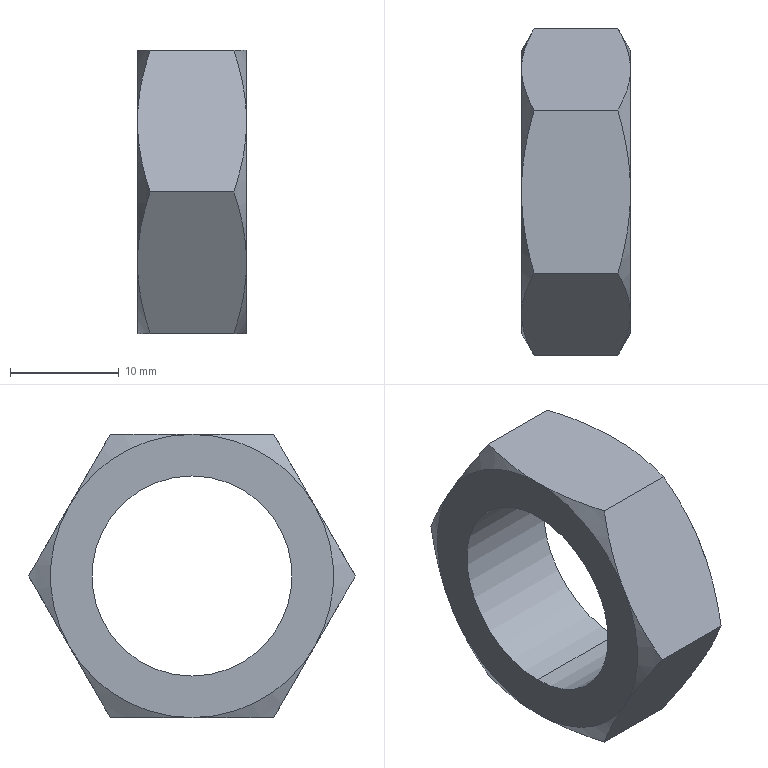Part | SolidWorks | features BaseBody 1 | 1 solid | 22 faces | box 10 x 30.022 x 26 mm | volume 3164 mm3 | cone 12 | plane 8 | cylinder 2 | commonest cylinder face diameters 18.376 x2
STEP:
#1=CARTESIAN_POINT('',(-65.,0.,9.188));
#2=VERTEX_POINT('',#1);
#3=CARTESIAN_POINT('',(-65.,0.,-9.188));
#4=VERTEX_POINT('',#3);
#5=CARTESIAN_POINT('',(-65.,0.,0.));
#6=DIRECTION('',(1.,0.,0.));
#7=DIRECTION('',(0.,0.,-1.));
#8=AXIS2_PLACEMENT_3D('',#5,#6,#7);
#9=CIRCLE('',#8,9.188);
#10=EDGE_CURVE('',#2,#4,#9,.T.);
#11=ORIENTED_EDGE('',*,*,#10,.F.);
#12=CARTESIAN_POINT('',(-55.,0.,9.188));
#13=VERTEX_POINT('',#12);
#14=CARTESIAN_POINT('',(-60.,0.,9.188));
#15=DIRECTION('',(1.,0.,0.));
#16=VECTOR('',#15,1000.);
#17=LINE('',#14,#16);
#18=EDGE_CURVE('',#2,#13,#17,.T.);
#19=ORIENTED_EDGE('',*,*,#18,.T.);
#20=CARTESIAN_POINT('',(-55.,0.,-9.188));
#21=VERTEX_POINT('',#20);
#22=CARTESIAN_POINT('',(-55.,0.,0.));
#23=DIRECTION('',(-1.,0.,0.));
#24=DIRECTION('',(0.,0.,-1.));
#25=AXIS2_PLACEMENT_3D('',#22,#23,#24);
#26=CIRCLE('',#25,9.188);
#27=EDGE_CURVE('',#21,#13,#26,.T.);
#28=ORIENTED_EDGE('',*,*,#27,.F.);
#29=CARTESIAN_POINT('',(-60.,0.,-9.188));
#30=DIRECTION('',(1.,0.,0.));
#31=VECTOR('',#30,1000.);
#32=LINE('',#29,#31);
#33=EDGE_CURVE('',#4,#21,#32,.T.);
#34=ORIENTED_EDGE('',*,*,#33,.F.);
#35=EDGE_LOOP('',(#11,#19,#28,#34));
#36=FACE_OUTER_BOUND('',#35,.T.);
#37=CARTESIAN_POINT('',(-60.,0.,0.));
#38=DIRECTION('',(1.,0.,0.));
#39=DIRECTION('',(0.,0.,-1.));
#40=AXIS2_PLACEMENT_3D('',#37,#38,#39);
#41=CYLINDRICAL_SURFACE('',#40,9.188);
#42=ADVANCED_FACE('',(#36),#41,.F.);
#43=ORIENTED_EDGE('',*,*,#18,.F.);
#44=CARTESIAN_POINT('',(-65.,0.,0.));
#45=DIRECTION('',(1.,0.,0.));
#46=DIRECTION('',(0.,0.,-1.));
#47=AXIS2_PLACEMENT_3D('',#44,#45,#46);
#48=CIRCLE('',#47,9.188);
#49=EDGE_CURVE('',#4,#2,#48,.T.);
#50=ORIENTED_EDGE('',*,*,#49,.F.);
#51=ORIENTED_EDGE('',*,*,#33,.T.);
#52=CARTESIAN_POINT('',(-55.,0.,0.));
#53=DIRECTION('',(-1.,0.,0.));
#54=DIRECTION('',(0.,0.,-1.));
#55=AXIS2_PLACEMENT_3D('',#52,#53,#54);
#56=CIRCLE('',#55,9.188);
#57=EDGE_CURVE('',#13,#21,#56,.T.);
#58=ORIENTED_EDGE('',*,*,#57,.F.);
#59=EDGE_LOOP('',(#43,#50,#51,#58));
#60=FACE_OUTER_BOUND('',#59,.T.);
#61=CARTESIAN_POINT('',(-60.,0.,0.));
#62=DIRECTION('',(1.,0.,0.));
#63=DIRECTION('',(0.,0.,-1.));
#64=AXIS2_PLACEMENT_3D('',#61,#62,#63);
#65=CYLINDRICAL_SURFACE('',#64,9.188);
#66=ADVANCED_FACE('',(#60),#65,.F.);
#67=ORIENTED_EDGE('',*,*,#27,.T.);
#68=ORIENTED_EDGE('',*,*,#57,.T.);
#69=EDGE_LOOP('',(#67,#68));
#70=FACE_BOUND('',#69,.T.);
#71=CARTESIAN_POINT('',(-55.,0.,13.));
#72=VERTEX_POINT('',#71);
#73=CARTESIAN_POINT('',(-55.,-11.258,6.5));
#74=VERTEX_POINT('',#73);
#75=CARTESIAN_POINT('',(-55.,0.,0.));
#76=DIRECTION('',(1.,0.,0.));
#77=DIRECTION('',(0.,0.,1.));
#78=AXIS2_PLACEMENT_3D('',#75,#76,#77);
#79=CIRCLE('',#78,13.);
#80=EDGE_CURVE('',#72,#74,#79,.T.);
#81=ORIENTED_EDGE('',*,*,#80,.T.);
#82=CARTESIAN_POINT('',(-55.,-11.258,-6.5));
#83=VERTEX_POINT('',#82);
#84=CARTESIAN_POINT('',(-55.,0.,0.));
#85=DIRECTION('',(1.,0.,0.));
#86=DIRECTION('',(0.,0.,1.));
#87=AXIS2_PLACEMENT_3D('',#84,#85,#86);
#88=CIRCLE('',#87,13.);
#89=EDGE_CURVE('',#74,#83,#88,.T.);
#90=ORIENTED_EDGE('',*,*,#89,.T.);
#91=CARTESIAN_POINT('',(-55.,0.,-13.));
#92=VERTEX_POINT('',#91);
#93=CARTESIAN_POINT('',(-55.,0.,0.));
#94=DIRECTION('',(1.,0.,0.));
#95=DIRECTION('',(0.,0.,1.));
#96=AXIS2_PLACEMENT_3D('',#93,#94,#95);
#97=CIRCLE('',#96,13.);
#98=EDGE_CURVE('',#83,#92,#97,.T.);
#99=ORIENTED_EDGE('',*,*,#98,.T.);
#100=CARTESIAN_POINT('',(-55.,11.258,-6.5));
#101=VERTEX_POINT('',#100);
#102=CARTESIAN_POINT('',(-55.,0.,0.));
#103=DIRECTION('',(1.,0.,0.));
#104=DIRECTION('',(0.,0.,1.));
#105=AXIS2_PLACEMENT_3D('',#102,#103,#104);
#106=CIRCLE('',#105,13.);
#107=EDGE_CURVE('',#92,#101,#106,.T.);
#108=ORIENTED_EDGE('',*,*,#107,.T.);
#109=CARTESIAN_POINT('',(-55.,11.258,6.5));
#110=VERTEX_POINT('',#109);
#111=CARTESIAN_POINT('',(-55.,0.,0.));
#112=DIRECTION('',(1.,0.,0.));
#113=DIRECTION('',(0.,0.,1.));
#114=AXIS2_PLACEMENT_3D('',#111,#112,#113);
#115=CIRCLE('',#114,13.);
#116=EDGE_CURVE('',#101,#110,#115,.T.);
#117=ORIENTED_EDGE('',*,*,#116,.T.);
#118=CARTESIAN_POINT('',(-55.,0.,0.));
#119=DIRECTION('',(1.,0.,0.));
#120=DIRECTION('',(0.,0.,1.));
#121=AXIS2_PLACEMENT_3D('',#118,#119,#120);
#122=CIRCLE('',#121,13.);
#123=EDGE_CURVE('',#110,#72,#122,.T.);
#124=ORIENTED_EDGE('',*,*,#123,.T.);
#125=EDGE_LOOP('',(#81,#90,#99,#108,#117,#124));
#126=FACE_OUTER_BOUND('',#125,.T.);
#127=CARTESIAN_POINT('',(-55.,-11.094,0.));
#128=DIRECTION('',(1.,0.,0.));
#129=DIRECTION('',(0.,0.,-1.));
#130=AXIS2_PLACEMENT_3D('',#127,#128,#129);
#131=PLANE('',#130);
#132=ADVANCED_FACE('',(#70,#126),#131,.T.);
#133=CARTESIAN_POINT('',(-65.,11.258,-6.5));
#134=VERTEX_POINT('',#133);
#135=CARTESIAN_POINT('',(-65.,0.,-13.));
#136=VERTEX_POINT('',#135);
#137=CARTESIAN_POINT('',(-65.,0.,0.));
#138=DIRECTION('',(-1.,0.,0.));
#139=DIRECTION('',(0.,0.,-1.));
#140=AXIS2_PLACEMENT_3D('',#137,#138,#139);
#141=CIRCLE('',#140,13.);
#142=EDGE_CURVE('',#134,#136,#141,.T.);
#143=ORIENTED_EDGE('',*,*,#142,.T.);
#144=CARTESIAN_POINT('',(-65.,-11.258,-6.5));
#145=VERTEX_POINT('',#144);
#146=CARTESIAN_POINT('',(-65.,0.,0.));
#147=DIRECTION('',(-1.,0.,0.));
#148=DIRECTION('',(0.,0.,-1.));
#149=AXIS2_PLACEMENT_3D('',#146,#147,#148);
#150=CIRCLE('',#149,13.);
#151=EDGE_CURVE('',#136,#145,#150,.T.);
#152=ORIENTED_EDGE('',*,*,#151,.T.);
#153=CARTESIAN_POINT('',(-65.,-11.258,6.5));
#154=VERTEX_POINT('',#153);
#155=CARTESIAN_POINT('',(-65.,0.,0.));
#156=DIRECTION('',(-1.,0.,0.));
#157=DIRECTION('',(0.,0.,-1.));
#158=AXIS2_PLACEMENT_3D('',#155,#156,#157);
#159=CIRCLE('',#158,13.);
#160=EDGE_CURVE('',#145,#154,#159,.T.);
#161=ORIENTED_EDGE('',*,*,#160,.T.);
#162=CARTESIAN_POINT('',(-65.,0.,13.));
#163=VERTEX_POINT('',#162);
#164=CARTESIAN_POINT('',(-65.,0.,0.));
#165=DIRECTION('',(-1.,0.,0.));
#166=DIRECTION('',(0.,0.,-1.));
#167=AXIS2_PLACEMENT_3D('',#164,#165,#166);
#168=CIRCLE('',#167,13.);
#169=EDGE_CURVE('',#154,#163,#168,.T.);
#170=ORIENTED_EDGE('',*,*,#169,.T.);
#171=CARTESIAN_POINT('',(-65.,11.258,6.5));
#172=VERTEX_POINT('',#171);
#173=CARTESIAN_POINT('',(-65.,0.,0.));
#174=DIRECTION('',(-1.,0.,0.));
#175=DIRECTION('',(0.,0.,-1.));
#176=AXIS2_PLACEMENT_3D('',#173,#174,#175);
#177=CIRCLE('',#176,13.);
#178=EDGE_CURVE('',#163,#172,#177,.T.);
#179=ORIENTED_EDGE('',*,*,#178,.T.);
#180=CARTESIAN_POINT('',(-65.,0.,0.));
#181=DIRECTION('',(-1.,0.,0.));
#182=DIRECTION('',(0.,0.,-1.));
#183=AXIS2_PLACEMENT_3D('',#180,#181,#182);
#184=CIRCLE('',#183,13.);
#185=EDGE_CURVE('',#172,#134,#184,.T.);
#186=ORIENTED_EDGE('',*,*,#185,.T.);
#187=EDGE_LOOP('',(#143,#152,#161,#170,#179,#186));
#188=FACE_OUTER_BOUND('',#187,.T.);
#189=ORIENTED_EDGE('',*,*,#49,.T.);
#190=ORIENTED_EDGE('',*,*,#10,.T.);
#191=EDGE_LOOP('',(#189,#190));
#192=FACE_BOUND('',#191,.T.);
#193=CARTESIAN_POINT('',(-65.,-11.094,0.));
#194=DIRECTION('',(-1.,0.,0.));
#195=DIRECTION('',(0.,0.,1.));
#196=AXIS2_PLACEMENT_3D('',#193,#194,#195);
#197=PLANE('',#196);
#198=ADVANCED_FACE('',(#188,#192),#197,.T.);
#199=ORIENTED_EDGE('',*,*,#89,.F.);
#200=CARTESIAN_POINT('',(-56.161,-15.011,0.));
#201=VERTEX_POINT('',#200);
#202=CARTESIAN_POINT('',(-55.,-11.258,6.5));
#203=CARTESIAN_POINT('',(-55.,-11.899,5.391));
#204=CARTESIAN_POINT('',(-55.111,-12.531,4.296));
#205=CARTESIAN_POINT('',(-55.515,-13.78,2.132));
#206=CARTESIAN_POINT('',(-55.807,-14.398,1.062));
#207=CARTESIAN_POINT('',(-56.161,-15.011,0.));
#208=B_SPLINE_CURVE_WITH_KNOTS('',3,(#202,#203,#204,#205,#206,#207),.UNSPECIFIED.,.F.,.F.,(4,2,4),(0.,0.003797,0.007595),.UNSPECIFIED.);
#209=EDGE_CURVE('',#74,#201,#208,.T.);
#210=ORIENTED_EDGE('',*,*,#209,.T.);
#211=CARTESIAN_POINT('',(-56.161,-15.011,0.));
#212=CARTESIAN_POINT('',(-55.807,-14.398,-1.062));
#213=CARTESIAN_POINT('',(-55.515,-13.78,-2.132));
#214=CARTESIAN_POINT('',(-55.111,-12.531,-4.296));
#215=CARTESIAN_POINT('',(-55.,-11.899,-5.391));
#216=CARTESIAN_POINT('',(-55.,-11.258,-6.5));
#217=B_SPLINE_CURVE_WITH_KNOTS('',3,(#211,#212,#213,#214,#215,#216),.UNSPECIFIED.,.F.,.F.,(4,2,4),(0.,0.003797,0.007595),.UNSPECIFIED.);
#218=EDGE_CURVE('',#201,#83,#217,.T.);
#219=ORIENTED_EDGE('',*,*,#218,.T.);
#220=EDGE_LOOP('',(#199,#210,#219));
#221=FACE_OUTER_BOUND('',#220,.T.);
#222=CARTESIAN_POINT('',(-56.168,0.,0.));
#223=DIRECTION('',(-1.,0.,0.));
#224=DIRECTION('',(0.,0.,1.));
#225=AXIS2_PLACEMENT_3D('',#222,#223,#224);
#226=CONICAL_SURFACE('',#225,15.023,1.047);
#227=ADVANCED_FACE('',(#221),#226,.T.);
#228=CARTESIAN_POINT('',(-56.161,-7.506,13.));
#229=VERTEX_POINT('',#228);
#230=CARTESIAN_POINT('',(-56.161,-7.506,13.));
#231=CARTESIAN_POINT('',(-55.807,-8.119,11.938));
#232=CARTESIAN_POINT('',(-55.515,-8.736,10.868));
#233=CARTESIAN_POINT('',(-55.111,-9.986,8.704));
#234=CARTESIAN_POINT('',(-55.,-10.618,7.609));
#235=CARTESIAN_POINT('',(-55.,-11.258,6.5));
#236=B_SPLINE_CURVE_WITH_KNOTS('',3,(#230,#231,#232,#233,#234,#235),.UNSPECIFIED.,.F.,.F.,(4,2,4),(0.,0.003797,0.007595),.UNSPECIFIED.);
#237=EDGE_CURVE('',#229,#74,#236,.T.);
#238=ORIENTED_EDGE('',*,*,#237,.T.);
#239=ORIENTED_EDGE('',*,*,#80,.F.);
#240=CARTESIAN_POINT('',(-55.,0.,13.));
#241=CARTESIAN_POINT('',(-55.,-1.281,13.));
#242=CARTESIAN_POINT('',(-55.111,-2.545,13.));
#243=CARTESIAN_POINT('',(-55.515,-5.044,13.));
#244=CARTESIAN_POINT('',(-55.807,-6.279,13.));
#245=CARTESIAN_POINT('',(-56.161,-7.506,13.));
#246=B_SPLINE_CURVE_WITH_KNOTS('',3,(#240,#241,#242,#243,#244,#245),.UNSPECIFIED.,.F.,.F.,(4,2,4),(0.,0.003797,0.007595),.UNSPECIFIED.);
#247=EDGE_CURVE('',#72,#229,#246,.T.);
#248=ORIENTED_EDGE('',*,*,#247,.T.);
#249=EDGE_LOOP('',(#238,#239,#248));
#250=FACE_OUTER_BOUND('',#249,.T.);
#251=CARTESIAN_POINT('',(-56.168,0.,0.));
#252=DIRECTION('',(-1.,0.,0.));
#253=DIRECTION('',(0.,0.,1.));
#254=AXIS2_PLACEMENT_3D('',#251,#252,#253);
#255=CONICAL_SURFACE('',#254,15.023,1.047);
#256=ADVANCED_FACE('',(#250),#255,.T.);
#257=CARTESIAN_POINT('',(-56.161,7.506,13.));
#258=VERTEX_POINT('',#257);
#259=CARTESIAN_POINT('',(-56.161,7.506,13.));
#260=CARTESIAN_POINT('',(-55.807,6.279,13.));
#261=CARTESIAN_POINT('',(-55.515,5.044,13.));
#262=CARTESIAN_POINT('',(-55.111,2.545,13.));
#263=CARTESIAN_POINT('',(-55.,1.281,13.));
#264=CARTESIAN_POINT('',(-55.,0.,13.));
#265=B_SPLINE_CURVE_WITH_KNOTS('',3,(#259,#260,#261,#262,#263,#264),.UNSPECIFIED.,.F.,.F.,(4,2,4),(0.,0.003797,0.007595),.UNSPECIFIED.);
#266=EDGE_CURVE('',#258,#72,#265,.T.);
#267=ORIENTED_EDGE('',*,*,#266,.T.);
#268=ORIENTED_EDGE('',*,*,#123,.F.);
#269=CARTESIAN_POINT('',(-55.,11.258,6.5));
#270=CARTESIAN_POINT('',(-55.,10.618,7.609));
#271=CARTESIAN_POINT('',(-55.111,9.986,8.704));
#272=CARTESIAN_POINT('',(-55.515,8.736,10.868));
#273=CARTESIAN_POINT('',(-55.807,8.119,11.938));
#274=CARTESIAN_POINT('',(-56.161,7.506,13.));
#275=B_SPLINE_CURVE_WITH_KNOTS('',3,(#269,#270,#271,#272,#273,#274),.UNSPECIFIED.,.F.,.F.,(4,2,4),(0.,0.003797,0.007595),.UNSPECIFIED.);
#276=EDGE_CURVE('',#110,#258,#275,.T.);
#277=ORIENTED_EDGE('',*,*,#276,.T.);
#278=EDGE_LOOP('',(#267,#268,#277));
#279=FACE_OUTER_BOUND('',#278,.T.);
#280=CARTESIAN_POINT('',(-56.168,0.,0.));
#281=DIRECTION('',(-1.,0.,0.));
#282=DIRECTION('',(0.,0.,1.));
#283=AXIS2_PLACEMENT_3D('',#280,#281,#282);
#284=CONICAL_SURFACE('',#283,15.023,1.047);
#285=ADVANCED_FACE('',(#279),#284,.T.);
#286=CARTESIAN_POINT('',(-56.161,15.011,0.));
#287=VERTEX_POINT('',#286);
#288=CARTESIAN_POINT('',(-56.161,15.011,0.));
#289=CARTESIAN_POINT('',(-55.807,14.398,1.062));
#290=CARTESIAN_POINT('',(-55.515,13.78,2.132));
#291=CARTESIAN_POINT('',(-55.111,12.531,4.296));
#292=CARTESIAN_POINT('',(-55.,11.899,5.391));
#293=CARTESIAN_POINT('',(-55.,11.258,6.5));
#294=B_SPLINE_CURVE_WITH_KNOTS('',3,(#288,#289,#290,#291,#292,#293),.UNSPECIFIED.,.F.,.F.,(4,2,4),(0.,0.003797,0.007595),.UNSPECIFIED.);
#295=EDGE_CURVE('',#287,#110,#294,.T.);
#296=ORIENTED_EDGE('',*,*,#295,.T.);
#297=ORIENTED_EDGE('',*,*,#116,.F.);
#298=CARTESIAN_POINT('',(-55.,11.258,-6.5));
#299=CARTESIAN_POINT('',(-55.,11.899,-5.391));
#300=CARTESIAN_POINT('',(-55.111,12.531,-4.296));
#301=CARTESIAN_POINT('',(-55.515,13.78,-2.132));
#302=CARTESIAN_POINT('',(-55.807,14.398,-1.062));
#303=CARTESIAN_POINT('',(-56.161,15.011,0.));
#304=B_SPLINE_CURVE_WITH_KNOTS('',3,(#298,#299,#300,#301,#302,#303),.UNSPECIFIED.,.F.,.F.,(4,2,4),(0.,0.003797,0.007595),.UNSPECIFIED.);
#305=EDGE_CURVE('',#101,#287,#304,.T.);
#306=ORIENTED_EDGE('',*,*,#305,.T.);
#307=EDGE_LOOP('',(#296,#297,#306));
#308=FACE_OUTER_BOUND('',#307,.T.);
#309=CARTESIAN_POINT('',(-56.168,0.,0.));
#310=DIRECTION('',(-1.,0.,0.));
#311=DIRECTION('',(0.,0.,1.));
#312=AXIS2_PLACEMENT_3D('',#309,#310,#311);
#313=CONICAL_SURFACE('',#312,15.023,1.047);
#314=ADVANCED_FACE('',(#308),#313,.T.);
#315=ORIENTED_EDGE('',*,*,#107,.F.);
#316=CARTESIAN_POINT('',(-56.161,7.506,-13.));
#317=VERTEX_POINT('',#316);
#318=CARTESIAN_POINT('',(-55.,0.,-13.));
#319=CARTESIAN_POINT('',(-55.,1.281,-13.));
#320=CARTESIAN_POINT('',(-55.111,2.545,-13.));
#321=CARTESIAN_POINT('',(-55.515,5.044,-13.));
#322=CARTESIAN_POINT('',(-55.807,6.279,-13.));
#323=CARTESIAN_POINT('',(-56.161,7.506,-13.));
#324=B_SPLINE_CURVE_WITH_KNOTS('',3,(#318,#319,#320,#321,#322,#323),.UNSPECIFIED.,.F.,.F.,(4,2,4),(0.,0.003797,0.007595),.UNSPECIFIED.);
#325=EDGE_CURVE('',#92,#317,#324,.T.);
#326=ORIENTED_EDGE('',*,*,#325,.T.);
#327=CARTESIAN_POINT('',(-56.161,7.506,-13.));
#328=CARTESIAN_POINT('',(-55.807,8.119,-11.938));
#329=CARTESIAN_POINT('',(-55.515,8.736,-10.868));
#330=CARTESIAN_POINT('',(-55.111,9.986,-8.704));
#331=CARTESIAN_POINT('',(-55.,10.618,-7.609));
#332=CARTESIAN_POINT('',(-55.,11.258,-6.5));
#333=B_SPLINE_CURVE_WITH_KNOTS('',3,(#327,#328,#329,#330,#331,#332),.UNSPECIFIED.,.F.,.F.,(4,2,4),(0.,0.003797,0.007595),.UNSPECIFIED.);
#334=EDGE_CURVE('',#317,#101,#333,.T.);
#335=ORIENTED_EDGE('',*,*,#334,.T.);
#336=EDGE_LOOP('',(#315,#326,#335));
#337=FACE_OUTER_BOUND('',#336,.T.);
#338=CARTESIAN_POINT('',(-56.168,0.,0.));
#339=DIRECTION('',(-1.,0.,0.));
#340=DIRECTION('',(0.,0.,1.));
#341=AXIS2_PLACEMENT_3D('',#338,#339,#340);
#342=CONICAL_SURFACE('',#341,15.023,1.047);
#343=ADVANCED_FACE('',(#337),#342,.T.);
#344=ORIENTED_EDGE('',*,*,#98,.F.);
#345=CARTESIAN_POINT('',(-56.161,-7.506,-13.));
#346=VERTEX_POINT('',#345);
#347=CARTESIAN_POINT('',(-55.,-11.258,-6.5));
#348=CARTESIAN_POINT('',(-55.,-10.618,-7.609));
#349=CARTESIAN_POINT('',(-55.111,-9.986,-8.704));
#350=CARTESIAN_POINT('',(-55.515,-8.736,-10.868));
#351=CARTESIAN_POINT('',(-55.807,-8.119,-11.938));
#352=CARTESIAN_POINT('',(-56.161,-7.506,-13.));
#353=B_SPLINE_CURVE_WITH_KNOTS('',3,(#347,#348,#349,#350,#351,#352),.UNSPECIFIED.,.F.,.F.,(4,2,4),(0.,0.003797,0.007595),.UNSPECIFIED.);
#354=EDGE_CURVE('',#83,#346,#353,.T.);
#355=ORIENTED_EDGE('',*,*,#354,.T.);
#356=CARTESIAN_POINT('',(-56.161,-7.506,-13.));
#357=CARTESIAN_POINT('',(-55.807,-6.279,-13.));
#358=CARTESIAN_POINT('',(-55.515,-5.044,-13.));
#359=CARTESIAN_POINT('',(-55.111,-2.545,-13.));
#360=CARTESIAN_POINT('',(-55.,-1.281,-13.));
#361=CARTESIAN_POINT('',(-55.,0.,-13.));
#362=B_SPLINE_CURVE_WITH_KNOTS('',3,(#356,#357,#358,#359,#360,#361),.UNSPECIFIED.,.F.,.F.,(4,2,4),(0.,0.003797,0.007595),.UNSPECIFIED.);
#363=EDGE_CURVE('',#346,#92,#362,.T.);
#364=ORIENTED_EDGE('',*,*,#363,.T.);
#365=EDGE_LOOP('',(#344,#355,#364));
#366=FACE_OUTER_BOUND('',#365,.T.);
#367=CARTESIAN_POINT('',(-56.168,0.,0.));
#368=DIRECTION('',(-1.,0.,0.));
#369=DIRECTION('',(0.,0.,1.));
#370=AXIS2_PLACEMENT_3D('',#367,#368,#369);
#371=CONICAL_SURFACE('',#370,15.023,1.047);
#372=ADVANCED_FACE('',(#366),#371,.T.);
#373=CARTESIAN_POINT('',(-63.839,-7.506,-13.));
#374=VERTEX_POINT('',#373);
#375=CARTESIAN_POINT('',(-63.839,-7.506,-13.));
#376=CARTESIAN_POINT('',(-64.193,-8.119,-11.938));
#377=CARTESIAN_POINT('',(-64.485,-8.736,-10.868));
#378=CARTESIAN_POINT('',(-64.889,-9.986,-8.704));
#379=CARTESIAN_POINT('',(-65.,-10.618,-7.609));
#380=CARTESIAN_POINT('',(-65.,-11.258,-6.5));
#381=B_SPLINE_CURVE_WITH_KNOTS('',3,(#375,#376,#377,#378,#379,#380),.UNSPECIFIED.,.F.,.F.,(4,2,4),(0.,0.003797,0.007595),.UNSPECIFIED.);
#382=EDGE_CURVE('',#374,#145,#381,.T.);
#383=ORIENTED_EDGE('',*,*,#382,.T.);
#384=ORIENTED_EDGE('',*,*,#151,.F.);
#385=CARTESIAN_POINT('',(-65.,0.,-13.));
#386=CARTESIAN_POINT('',(-65.,-1.281,-13.));
#387=CARTESIAN_POINT('',(-64.889,-2.545,-13.));
#388=CARTESIAN_POINT('',(-64.485,-5.044,-13.));
#389=CARTESIAN_POINT('',(-64.193,-6.279,-13.));
#390=CARTESIAN_POINT('',(-63.839,-7.506,-13.));
#391=B_SPLINE_CURVE_WITH_KNOTS('',3,(#385,#386,#387,#388,#389,#390),.UNSPECIFIED.,.F.,.F.,(4,2,4),(0.,0.003797,0.007595),.UNSPECIFIED.);
#392=EDGE_CURVE('',#136,#374,#391,.T.);
#393=ORIENTED_EDGE('',*,*,#392,.T.);
#394=EDGE_LOOP('',(#383,#384,#393));
#395=FACE_OUTER_BOUND('',#394,.T.);
#396=CARTESIAN_POINT('',(-63.832,0.,0.));
#397=DIRECTION('',(1.,0.,0.));
#398=DIRECTION('',(0.,0.,-1.));
#399=AXIS2_PLACEMENT_3D('',#396,#397,#398);
#400=CONICAL_SURFACE('',#399,15.023,1.047);
#401=ADVANCED_FACE('',(#395),#400,.T.);
#402=ORIENTED_EDGE('',*,*,#142,.F.);
#403=CARTESIAN_POINT('',(-63.839,7.506,-13.));
#404=VERTEX_POINT('',#403);
#405=CARTESIAN_POINT('',(-65.,11.258,-6.5));
#406=CARTESIAN_POINT('',(-65.,10.618,-7.609));
#407=CARTESIAN_POINT('',(-64.889,9.986,-8.704));
#408=CARTESIAN_POINT('',(-64.485,8.736,-10.868));
#409=CARTESIAN_POINT('',(-64.193,8.119,-11.938));
#410=CARTESIAN_POINT('',(-63.839,7.506,-13.));
#411=B_SPLINE_CURVE_WITH_KNOTS('',3,(#405,#406,#407,#408,#409,#410),.UNSPECIFIED.,.F.,.F.,(4,2,4),(0.,0.003797,0.007595),.UNSPECIFIED.);
#412=EDGE_CURVE('',#134,#404,#411,.T.);
#413=ORIENTED_EDGE('',*,*,#412,.T.);
#414=CARTESIAN_POINT('',(-63.839,7.506,-13.));
#415=CARTESIAN_POINT('',(-64.193,6.279,-13.));
#416=CARTESIAN_POINT('',(-64.485,5.044,-13.));
#417=CARTESIAN_POINT('',(-64.889,2.545,-13.));
#418=CARTESIAN_POINT('',(-65.,1.281,-13.));
#419=CARTESIAN_POINT('',(-65.,0.,-13.));
#420=B_SPLINE_CURVE_WITH_KNOTS('',3,(#414,#415,#416,#417,#418,#419),.UNSPECIFIED.,.F.,.F.,(4,2,4),(0.,0.003797,0.007595),.UNSPECIFIED.);
#421=EDGE_CURVE('',#404,#136,#420,.T.);
#422=ORIENTED_EDGE('',*,*,#421,.T.);
#423=EDGE_LOOP('',(#402,#413,#422));
#424=FACE_OUTER_BOUND('',#423,.T.);
#425=CARTESIAN_POINT('',(-63.832,0.,0.));
#426=DIRECTION('',(1.,0.,0.));
#427=DIRECTION('',(0.,0.,-1.));
#428=AXIS2_PLACEMENT_3D('',#425,#426,#427);
#429=CONICAL_SURFACE('',#428,15.023,1.047);
#430=ADVANCED_FACE('',(#424),#429,.T.);
#431=CARTESIAN_POINT('',(-63.839,15.011,0.));
#432=VERTEX_POINT('',#431);
#433=CARTESIAN_POINT('',(-63.839,15.011,0.));
#434=CARTESIAN_POINT('',(-64.193,14.398,-1.062));
#435=CARTESIAN_POINT('',(-64.485,13.78,-2.132));
#436=CARTESIAN_POINT('',(-64.889,12.531,-4.296));
#437=CARTESIAN_POINT('',(-65.,11.899,-5.391));
#438=CARTESIAN_POINT('',(-65.,11.258,-6.5));
#439=B_SPLINE_CURVE_WITH_KNOTS('',3,(#433,#434,#435,#436,#437,#438),.UNSPECIFIED.,.F.,.F.,(4,2,4),(0.,0.003797,0.007595),.UNSPECIFIED.);
#440=EDGE_CURVE('',#432,#134,#439,.T.);
#441=ORIENTED_EDGE('',*,*,#440,.T.);
#442=ORIENTED_EDGE('',*,*,#185,.F.);
#443=CARTESIAN_POINT('',(-65.,11.258,6.5));
#444=CARTESIAN_POINT('',(-65.,11.899,5.391));
#445=CARTESIAN_POINT('',(-64.889,12.531,4.296));
#446=CARTESIAN_POINT('',(-64.485,13.78,2.132));
#447=CARTESIAN_POINT('',(-64.193,14.398,1.062));
#448=CARTESIAN_POINT('',(-63.839,15.011,0.));
#449=B_SPLINE_CURVE_WITH_KNOTS('',3,(#443,#444,#445,#446,#447,#448),.UNSPECIFIED.,.F.,.F.,(4,2,4),(0.,0.003797,0.007595),.UNSPECIFIED.);
#450=EDGE_CURVE('',#172,#432,#449,.T.);
#451=ORIENTED_EDGE('',*,*,#450,.T.);
#452=EDGE_LOOP('',(#441,#442,#451));
#453=FACE_OUTER_BOUND('',#452,.T.);
#454=CARTESIAN_POINT('',(-63.832,0.,0.));
#455=DIRECTION('',(1.,0.,0.));
#456=DIRECTION('',(0.,0.,-1.));
#457=AXIS2_PLACEMENT_3D('',#454,#455,#456);
#458=CONICAL_SURFACE('',#457,15.023,1.047);
#459=ADVANCED_FACE('',(#453),#458,.T.);
#460=ORIENTED_EDGE('',*,*,#178,.F.);
#461=CARTESIAN_POINT('',(-63.839,7.506,13.));
#462=VERTEX_POINT('',#461);
#463=CARTESIAN_POINT('',(-65.,0.,13.));
#464=CARTESIAN_POINT('',(-65.,1.281,13.));
#465=CARTESIAN_POINT('',(-64.889,2.545,13.));
#466=CARTESIAN_POINT('',(-64.485,5.044,13.));
#467=CARTESIAN_POINT('',(-64.193,6.279,13.));
#468=CARTESIAN_POINT('',(-63.839,7.506,13.));
#469=B_SPLINE_CURVE_WITH_KNOTS('',3,(#463,#464,#465,#466,#467,#468),.UNSPECIFIED.,.F.,.F.,(4,2,4),(0.,0.003797,0.007595),.UNSPECIFIED.);
#470=EDGE_CURVE('',#163,#462,#469,.T.);
#471=ORIENTED_EDGE('',*,*,#470,.T.);
#472=CARTESIAN_POINT('',(-63.839,7.506,13.));
#473=CARTESIAN_POINT('',(-64.193,8.119,11.938));
#474=CARTESIAN_POINT('',(-64.485,8.736,10.868));
#475=CARTESIAN_POINT('',(-64.889,9.986,8.704));
#476=CARTESIAN_POINT('',(-65.,10.618,7.609));
#477=CARTESIAN_POINT('',(-65.,11.258,6.5));
#478=B_SPLINE_CURVE_WITH_KNOTS('',3,(#472,#473,#474,#475,#476,#477),.UNSPECIFIED.,.F.,.F.,(4,2,4),(0.,0.003797,0.007595),.UNSPECIFIED.);
#479=EDGE_CURVE('',#462,#172,#478,.T.);
#480=ORIENTED_EDGE('',*,*,#479,.T.);
#481=EDGE_LOOP('',(#460,#471,#480));
#482=FACE_OUTER_BOUND('',#481,.T.);
#483=CARTESIAN_POINT('',(-63.832,0.,0.));
#484=DIRECTION('',(1.,0.,0.));
#485=DIRECTION('',(0.,0.,-1.));
#486=AXIS2_PLACEMENT_3D('',#483,#484,#485);
#487=CONICAL_SURFACE('',#486,15.023,1.047);
#488=ADVANCED_FACE('',(#482),#487,.T.);
#489=CARTESIAN_POINT('',(-63.839,-7.506,13.));
#490=VERTEX_POINT('',#489);
#491=CARTESIAN_POINT('',(-63.839,-7.506,13.));
#492=CARTESIAN_POINT('',(-64.193,-6.279,13.));
#493=CARTESIAN_POINT('',(-64.485,-5.044,13.));
#494=CARTESIAN_POINT('',(-64.889,-2.545,13.));
#495=CARTESIAN_POINT('',(-65.,-1.281,13.));
#496=CARTESIAN_POINT('',(-65.,0.,13.));
#497=B_SPLINE_CURVE_WITH_KNOTS('',3,(#491,#492,#493,#494,#495,#496),.UNSPECIFIED.,.F.,.F.,(4,2,4),(0.,0.003797,0.007595),.UNSPECIFIED.);
#498=EDGE_CURVE('',#490,#163,#497,.T.);
#499=ORIENTED_EDGE('',*,*,#498,.T.);
#500=ORIENTED_EDGE('',*,*,#169,.F.);
#501=CARTESIAN_POINT('',(-65.,-11.258,6.5));
#502=CARTESIAN_POINT('',(-65.,-10.618,7.609));
#503=CARTESIAN_POINT('',(-64.889,-9.986,8.704));
#504=CARTESIAN_POINT('',(-64.485,-8.736,10.868));
#505=CARTESIAN_POINT('',(-64.193,-8.119,11.938));
#506=CARTESIAN_POINT('',(-63.839,-7.506,13.));
#507=B_SPLINE_CURVE_WITH_KNOTS('',3,(#501,#502,#503,#504,#505,#506),.UNSPECIFIED.,.F.,.F.,(4,2,4),(0.,0.003797,0.007595),.UNSPECIFIED.);
#508=EDGE_CURVE('',#154,#490,#507,.T.);
#509=ORIENTED_EDGE('',*,*,#508,.T.);
#510=EDGE_LOOP('',(#499,#500,#509));
#511=FACE_OUTER_BOUND('',#510,.T.);
#512=CARTESIAN_POINT('',(-63.832,0.,0.));
#513=DIRECTION('',(1.,0.,0.));
#514=DIRECTION('',(0.,0.,-1.));
#515=AXIS2_PLACEMENT_3D('',#512,#513,#514);
#516=CONICAL_SURFACE('',#515,15.023,1.047);
#517=ADVANCED_FACE('',(#511),#516,.T.);
#518=CARTESIAN_POINT('',(-63.839,-15.011,0.));
#519=VERTEX_POINT('',#518);
#520=CARTESIAN_POINT('',(-63.839,-15.011,0.));
#521=CARTESIAN_POINT('',(-64.193,-14.398,1.062));
#522=CARTESIAN_POINT('',(-64.485,-13.78,2.132));
#523=CARTESIAN_POINT('',(-64.889,-12.531,4.296));
#524=CARTESIAN_POINT('',(-65.,-11.899,5.391));
#525=CARTESIAN_POINT('',(-65.,-11.258,6.5));
#526=B_SPLINE_CURVE_WITH_KNOTS('',3,(#520,#521,#522,#523,#524,#525),.UNSPECIFIED.,.F.,.F.,(4,2,4),(0.,0.003797,0.007595),.UNSPECIFIED.);
#527=EDGE_CURVE('',#519,#154,#526,.T.);
#528=ORIENTED_EDGE('',*,*,#527,.T.);
#529=ORIENTED_EDGE('',*,*,#160,.F.);
#530=CARTESIAN_POINT('',(-65.,-11.258,-6.5));
#531=CARTESIAN_POINT('',(-65.,-11.899,-5.391));
#532=CARTESIAN_POINT('',(-64.889,-12.531,-4.296));
#533=CARTESIAN_POINT('',(-64.485,-13.78,-2.132));
#534=CARTESIAN_POINT('',(-64.193,-14.398,-1.062));
#535=CARTESIAN_POINT('',(-63.839,-15.011,0.));
#536=B_SPLINE_CURVE_WITH_KNOTS('',3,(#530,#531,#532,#533,#534,#535),.UNSPECIFIED.,.F.,.F.,(4,2,4),(0.,0.003797,0.007595),.UNSPECIFIED.);
#537=EDGE_CURVE('',#145,#519,#536,.T.);
#538=ORIENTED_EDGE('',*,*,#537,.T.);
#539=EDGE_LOOP('',(#528,#529,#538));
#540=FACE_OUTER_BOUND('',#539,.T.);
#541=CARTESIAN_POINT('',(-63.832,0.,0.));
#542=DIRECTION('',(1.,0.,0.));
#543=DIRECTION('',(0.,0.,-1.));
#544=AXIS2_PLACEMENT_3D('',#541,#542,#543);
#545=CONICAL_SURFACE('',#544,15.023,1.047);
#546=ADVANCED_FACE('',(#540),#545,.T.);
#547=CARTESIAN_POINT('',(-55.,-15.011,0.));
#548=DIRECTION('',(-1.,0.,0.));
#549=VECTOR('',#548,1000.);
#550=LINE('',#547,#549);
#551=EDGE_CURVE('',#201,#519,#550,.T.);
#552=ORIENTED_EDGE('',*,*,#551,.F.);
#553=ORIENTED_EDGE('',*,*,#209,.F.);
#554=ORIENTED_EDGE('',*,*,#237,.F.);
#555=CARTESIAN_POINT('',(-55.,-7.506,13.));
#556=DIRECTION('',(1.,0.,0.));
#557=VECTOR('',#556,1000.);
#558=LINE('',#555,#557);
#559=EDGE_CURVE('',#490,#229,#558,.T.);
#560=ORIENTED_EDGE('',*,*,#559,.F.);
#561=ORIENTED_EDGE('',*,*,#508,.F.);
#562=ORIENTED_EDGE('',*,*,#527,.F.);
#563=EDGE_LOOP('',(#552,#553,#554,#560,#561,#562));
#564=FACE_OUTER_BOUND('',#563,.T.);
#565=CARTESIAN_POINT('',(-55.,-15.011,0.));
#566=DIRECTION('',(0.,0.866,-0.5));
#567=DIRECTION('',(0.,0.5,0.866));
#568=AXIS2_PLACEMENT_3D('',#565,#566,#567);
#569=PLANE('',#568);
#570=ADVANCED_FACE('',(#564),#569,.F.);
#571=ORIENTED_EDGE('',*,*,#498,.F.);
#572=ORIENTED_EDGE('',*,*,#559,.T.);
#573=ORIENTED_EDGE('',*,*,#247,.F.);
#574=ORIENTED_EDGE('',*,*,#266,.F.);
#575=CARTESIAN_POINT('',(-55.,7.506,13.));
#576=DIRECTION('',(1.,0.,0.));
#577=VECTOR('',#576,1000.);
#578=LINE('',#575,#577);
#579=EDGE_CURVE('',#462,#258,#578,.T.);
#580=ORIENTED_EDGE('',*,*,#579,.F.);
#581=ORIENTED_EDGE('',*,*,#470,.F.);
#582=EDGE_LOOP('',(#571,#572,#573,#574,#580,#581));
#583=FACE_OUTER_BOUND('',#582,.T.);
#584=CARTESIAN_POINT('',(-55.,-7.506,13.));
#585=DIRECTION('',(0.,0.,-1.));
#586=DIRECTION('',(-1.,0.,0.));
#587=AXIS2_PLACEMENT_3D('',#584,#585,#586);
#588=PLANE('',#587);
#589=ADVANCED_FACE('',(#583),#588,.F.);
#590=ORIENTED_EDGE('',*,*,#479,.F.);
#591=ORIENTED_EDGE('',*,*,#579,.T.);
#592=ORIENTED_EDGE('',*,*,#276,.F.);
#593=ORIENTED_EDGE('',*,*,#295,.F.);
#594=CARTESIAN_POINT('',(-55.,15.011,0.));
#595=DIRECTION('',(1.,0.,0.));
#596=VECTOR('',#595,1000.);
#597=LINE('',#594,#596);
#598=EDGE_CURVE('',#432,#287,#597,.T.);
#599=ORIENTED_EDGE('',*,*,#598,.F.);
#600=ORIENTED_EDGE('',*,*,#450,.F.);
#601=EDGE_LOOP('',(#590,#591,#592,#593,#599,#600));
#602=FACE_OUTER_BOUND('',#601,.T.);
#603=CARTESIAN_POINT('',(-55.,7.506,13.));
#604=DIRECTION('',(0.,-0.866,-0.5));
#605=DIRECTION('',(0.,0.5,-0.866));
#606=AXIS2_PLACEMENT_3D('',#603,#604,#605);
#607=PLANE('',#606);
#608=ADVANCED_FACE('',(#602),#607,.F.);
#609=ORIENTED_EDGE('',*,*,#440,.F.);
#610=ORIENTED_EDGE('',*,*,#598,.T.);
#611=ORIENTED_EDGE('',*,*,#305,.F.);
#612=ORIENTED_EDGE('',*,*,#334,.F.);
#613=CARTESIAN_POINT('',(-55.,7.506,-13.));
#614=DIRECTION('',(1.,0.,0.));
#615=VECTOR('',#614,1000.);
#616=LINE('',#613,#615);
#617=EDGE_CURVE('',#404,#317,#616,.T.);
#618=ORIENTED_EDGE('',*,*,#617,.F.);
#619=ORIENTED_EDGE('',*,*,#412,.F.);
#620=EDGE_LOOP('',(#609,#610,#611,#612,#618,#619));
#621=FACE_OUTER_BOUND('',#620,.T.);
#622=CARTESIAN_POINT('',(-55.,15.011,0.));
#623=DIRECTION('',(0.,-0.866,0.5));
#624=DIRECTION('',(0.,-0.5,-0.866));
#625=AXIS2_PLACEMENT_3D('',#622,#623,#624);
#626=PLANE('',#625);
#627=ADVANCED_FACE('',(#621),#626,.F.);
#628=ORIENTED_EDGE('',*,*,#617,.T.);
#629=ORIENTED_EDGE('',*,*,#325,.F.);
#630=ORIENTED_EDGE('',*,*,#363,.F.);
#631=CARTESIAN_POINT('',(-55.,-7.506,-13.));
#632=DIRECTION('',(1.,0.,0.));
#633=VECTOR('',#632,1000.);
#634=LINE('',#631,#633);
#635=EDGE_CURVE('',#374,#346,#634,.T.);
#636=ORIENTED_EDGE('',*,*,#635,.F.);
#637=ORIENTED_EDGE('',*,*,#392,.F.);
#638=ORIENTED_EDGE('',*,*,#421,.F.);
#639=EDGE_LOOP('',(#628,#629,#630,#636,#637,#638));
#640=FACE_OUTER_BOUND('',#639,.T.);
#641=CARTESIAN_POINT('',(-55.,7.506,-13.));
#642=DIRECTION('',(0.,0.,1.));
#643=DIRECTION('',(1.,0.,0.));
#644=AXIS2_PLACEMENT_3D('',#641,#642,#643);
#645=PLANE('',#644);
#646=ADVANCED_FACE('',(#640),#645,.F.);
#647=ORIENTED_EDGE('',*,*,#635,.T.);
#648=ORIENTED_EDGE('',*,*,#354,.F.);
#649=ORIENTED_EDGE('',*,*,#218,.F.);
#650=ORIENTED_EDGE('',*,*,#551,.T.);
#651=ORIENTED_EDGE('',*,*,#537,.F.);
#652=ORIENTED_EDGE('',*,*,#382,.F.);
#653=EDGE_LOOP('',(#647,#648,#649,#650,#651,#652));
#654=FACE_OUTER_BOUND('',#653,.T.);
#655=CARTESIAN_POINT('',(-55.,-7.506,-13.));
#656=DIRECTION('',(0.,0.866,0.5));
#657=DIRECTION('',(0.,-0.5,0.866));
#658=AXIS2_PLACEMENT_3D('',#655,#656,#657);
#659=PLANE('',#658);
#660=ADVANCED_FACE('',(#654),#659,.F.);
#661=CLOSED_SHELL('',(#42,#66,#132,#198,#227,#256,#285,#314,#343,#372,#401,#430,#459,#488,#517,#546,#570,#589,#608,#627,#646,#660));
#662=MANIFOLD_SOLID_BREP('',#661);
#663=CARTESIAN_POINT('',(0.,0.,0.));
#664=DIRECTION('',(0.,0.,1.));
#665=DIRECTION('',(1.,0.,0.));
#666=AXIS2_PLACEMENT_3D('',#663,#664,#665);
#667=(LENGTH_UNIT()NAMED_UNIT(*)SI_UNIT(.MILLI.,.METRE.));
#668=UNCERTAINTY_MEASURE_WITH_UNIT(LENGTH_MEASURE(0.00001),#667,'','');
#669=(NAMED_UNIT(*)PLANE_ANGLE_UNIT()SI_UNIT($,.RADIAN.));
#670=(NAMED_UNIT(*)SI_UNIT($,.STERADIAN.)SOLID_ANGLE_UNIT());
#671=(GEOMETRIC_REPRESENTATION_CONTEXT(3)GLOBAL_UNCERTAINTY_ASSIGNED_CONTEXT((#668))GLOBAL_UNIT_ASSIGNED_CONTEXT((#667,#669,#670))REPRESENTATION_CONTEXT('',''));
#672=ADVANCED_BREP_SHAPE_REPRESENTATION('',(#662,#666),#671);